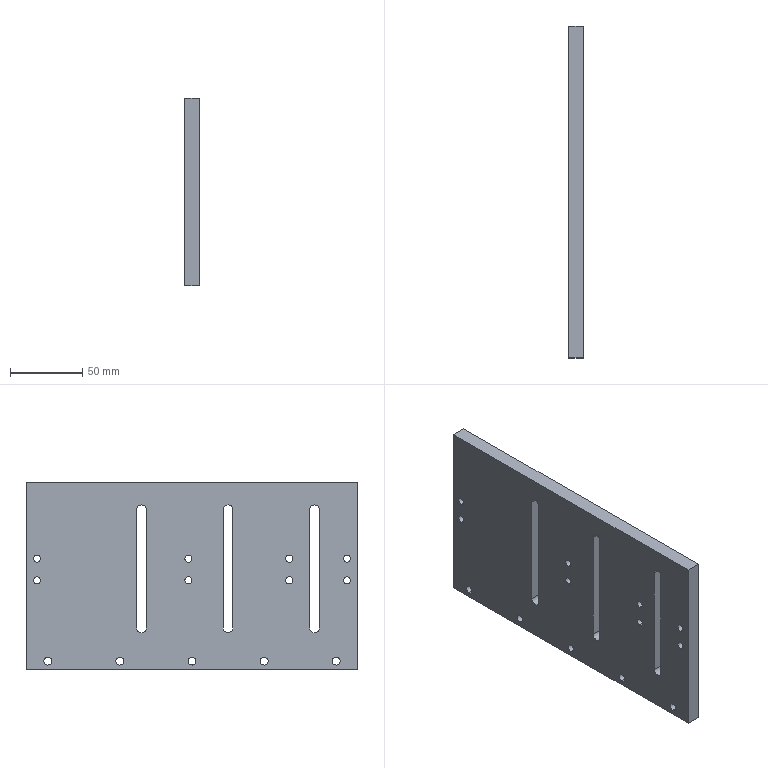Part | SolidWorks | features LPattern 6, HoleWzd 2, Extrusion 1, ICE 1 | 1 solid | 62 faces | box 10 x 230 x 130 mm | volume 277609 mm3 | cylinder 45 | plane 17 | commonest cylinder face diameters 5 x16 5.5 x10 10 x10 6.6 x9